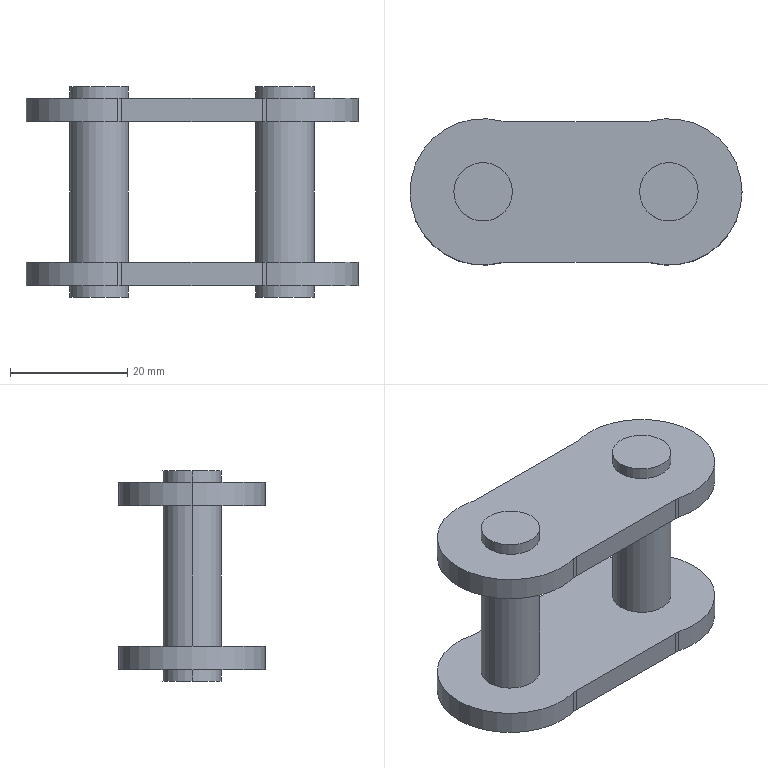Part | STEP file | Motor output chain-06B link 2 | 1 solid | 38 faces | box 56.75 x 25 x 36 mm | volume 14459 mm3 | cylinder 26 | plane 12 | commonest cylinder face diameters 10 x12 6 x8 25 x6
STEP:
#1=CARTESIAN_POINT('',(-20.875,0.,-16.));
#2=VERTEX_POINT('',#1);
#3=CARTESIAN_POINT('',(-10.875,0.,-16.));
#4=VERTEX_POINT('',#3);
#5=CARTESIAN_POINT('',(-15.875,0.,-16.));
#6=DIRECTION('',(0.,0.,-1.));
#7=DIRECTION('',(-1.,0.,0.));
#8=AXIS2_PLACEMENT_3D('',#5,#6,#7);
#9=CIRCLE('',#8,5.);
#10=EDGE_CURVE('',#2,#4,#9,.T.);
#11=ORIENTED_EDGE('',*,*,#10,.T.);
#12=CARTESIAN_POINT('',(-10.875,0.,-18.));
#13=VERTEX_POINT('',#12);
#14=CARTESIAN_POINT('',(-10.875,0.,18.));
#15=DIRECTION('',(0.,0.,-1.));
#16=VECTOR('',#15,1000.);
#17=LINE('',#14,#16);
#18=EDGE_CURVE('',#4,#13,#17,.T.);
#19=ORIENTED_EDGE('',*,*,#18,.T.);
#20=CARTESIAN_POINT('',(-20.875,0.,-18.));
#21=VERTEX_POINT('',#20);
#22=CARTESIAN_POINT('',(-15.875,0.,-18.));
#23=DIRECTION('',(0.,0.,1.));
#24=DIRECTION('',(1.,0.,0.));
#25=AXIS2_PLACEMENT_3D('',#22,#23,#24);
#26=CIRCLE('',#25,5.);
#27=EDGE_CURVE('',#13,#21,#26,.T.);
#28=ORIENTED_EDGE('',*,*,#27,.T.);
#29=CARTESIAN_POINT('',(-20.875,0.,18.));
#30=DIRECTION('',(0.,0.,-1.));
#31=VECTOR('',#30,1000.);
#32=LINE('',#29,#31);
#33=EDGE_CURVE('',#2,#21,#32,.T.);
#34=ORIENTED_EDGE('',*,*,#33,.F.);
#35=EDGE_LOOP('',(#11,#19,#28,#34));
#36=FACE_OUTER_BOUND('',#35,.T.);
#37=CARTESIAN_POINT('',(-15.875,0.,18.));
#38=DIRECTION('',(0.,0.,-1.));
#39=DIRECTION('',(-1.,0.,0.));
#40=AXIS2_PLACEMENT_3D('',#37,#38,#39);
#41=CYLINDRICAL_SURFACE('',#40,5.);
#42=ADVANCED_FACE('',(#36),#41,.T.);
#43=CARTESIAN_POINT('',(10.875,0.,-16.));
#44=VERTEX_POINT('',#43);
#45=CARTESIAN_POINT('',(20.875,0.,-16.));
#46=VERTEX_POINT('',#45);
#47=CARTESIAN_POINT('',(15.875,0.,-16.));
#48=DIRECTION('',(0.,0.,-1.));
#49=DIRECTION('',(-1.,0.,0.));
#50=AXIS2_PLACEMENT_3D('',#47,#48,#49);
#51=CIRCLE('',#50,5.);
#52=EDGE_CURVE('',#44,#46,#51,.T.);
#53=ORIENTED_EDGE('',*,*,#52,.T.);
#54=CARTESIAN_POINT('',(20.875,0.,-18.));
#55=VERTEX_POINT('',#54);
#56=CARTESIAN_POINT('',(20.875,0.,18.));
#57=DIRECTION('',(0.,0.,-1.));
#58=VECTOR('',#57,1000.);
#59=LINE('',#56,#58);
#60=EDGE_CURVE('',#46,#55,#59,.T.);
#61=ORIENTED_EDGE('',*,*,#60,.T.);
#62=CARTESIAN_POINT('',(10.875,0.,-18.));
#63=VERTEX_POINT('',#62);
#64=CARTESIAN_POINT('',(15.875,0.,-18.));
#65=DIRECTION('',(0.,0.,1.));
#66=DIRECTION('',(1.,0.,0.));
#67=AXIS2_PLACEMENT_3D('',#64,#65,#66);
#68=CIRCLE('',#67,5.);
#69=EDGE_CURVE('',#55,#63,#68,.T.);
#70=ORIENTED_EDGE('',*,*,#69,.T.);
#71=CARTESIAN_POINT('',(10.875,0.,18.));
#72=DIRECTION('',(0.,0.,-1.));
#73=VECTOR('',#72,1000.);
#74=LINE('',#71,#73);
#75=EDGE_CURVE('',#44,#63,#74,.T.);
#76=ORIENTED_EDGE('',*,*,#75,.F.);
#77=EDGE_LOOP('',(#53,#61,#70,#76));
#78=FACE_OUTER_BOUND('',#77,.T.);
#79=CARTESIAN_POINT('',(15.875,0.,18.));
#80=DIRECTION('',(0.,0.,-1.));
#81=DIRECTION('',(-1.,0.,0.));
#82=AXIS2_PLACEMENT_3D('',#79,#80,#81);
#83=CYLINDRICAL_SURFACE('',#82,5.);
#84=ADVANCED_FACE('',(#78),#83,.T.);
#85=CARTESIAN_POINT('',(12.726,-12.097,-16.));
#86=VERTEX_POINT('',#85);
#87=CARTESIAN_POINT('',(28.375,0.,-16.));
#88=VERTEX_POINT('',#87);
#89=CARTESIAN_POINT('',(15.875,0.,-16.));
#90=DIRECTION('',(0.,0.,1.));
#91=DIRECTION('',(1.,0.,0.));
#92=AXIS2_PLACEMENT_3D('',#89,#90,#91);
#93=CIRCLE('',#92,12.5);
#94=EDGE_CURVE('',#86,#88,#93,.T.);
#95=ORIENTED_EDGE('',*,*,#94,.T.);
#96=CARTESIAN_POINT('',(28.375,0.,-12.));
#97=VERTEX_POINT('',#96);
#98=CARTESIAN_POINT('',(28.375,0.,-16.));
#99=DIRECTION('',(0.,0.,1.));
#100=VECTOR('',#99,1000.);
#101=LINE('',#98,#100);
#102=EDGE_CURVE('',#88,#97,#101,.T.);
#103=ORIENTED_EDGE('',*,*,#102,.T.);
#104=CARTESIAN_POINT('',(12.726,-12.097,-12.));
#105=VERTEX_POINT('',#104);
#106=CARTESIAN_POINT('',(15.875,0.,-12.));
#107=DIRECTION('',(0.,0.,1.));
#108=DIRECTION('',(1.,0.,0.));
#109=AXIS2_PLACEMENT_3D('',#106,#107,#108);
#110=CIRCLE('',#109,12.5);
#111=EDGE_CURVE('',#105,#97,#110,.T.);
#112=ORIENTED_EDGE('',*,*,#111,.F.);
#113=CARTESIAN_POINT('',(12.726,-12.097,-16.));
#114=DIRECTION('',(0.,0.,1.));
#115=VECTOR('',#114,1000.);
#116=LINE('',#113,#115);
#117=EDGE_CURVE('',#86,#105,#116,.T.);
#118=ORIENTED_EDGE('',*,*,#117,.F.);
#119=EDGE_LOOP('',(#95,#103,#112,#118));
#120=FACE_OUTER_BOUND('',#119,.T.);
#121=CARTESIAN_POINT('',(15.875,0.,-16.));
#122=DIRECTION('',(0.,0.,1.));
#123=DIRECTION('',(1.,0.,0.));
#124=AXIS2_PLACEMENT_3D('',#121,#122,#123);
#125=CYLINDRICAL_SURFACE('',#124,12.5);
#126=ADVANCED_FACE('',(#120),#125,.T.);
#127=CARTESIAN_POINT('',(20.875,0.,18.));
#128=VERTEX_POINT('',#127);
#129=CARTESIAN_POINT('',(10.875,0.,18.));
#130=VERTEX_POINT('',#129);
#131=CARTESIAN_POINT('',(15.875,0.,18.));
#132=DIRECTION('',(0.,0.,1.));
#133=DIRECTION('',(1.,0.,0.));
#134=AXIS2_PLACEMENT_3D('',#131,#132,#133);
#135=CIRCLE('',#134,5.);
#136=EDGE_CURVE('',#128,#130,#135,.T.);
#137=ORIENTED_EDGE('',*,*,#136,.F.);
#138=CARTESIAN_POINT('',(20.875,0.,16.));
#139=VERTEX_POINT('',#138);
#140=CARTESIAN_POINT('',(20.875,0.,18.));
#141=DIRECTION('',(0.,0.,-1.));
#142=VECTOR('',#141,1000.);
#143=LINE('',#140,#142);
#144=EDGE_CURVE('',#128,#139,#143,.T.);
#145=ORIENTED_EDGE('',*,*,#144,.T.);
#146=CARTESIAN_POINT('',(10.875,0.,16.));
#147=VERTEX_POINT('',#146);
#148=CARTESIAN_POINT('',(15.875,0.,16.));
#149=DIRECTION('',(0.,0.,-1.));
#150=DIRECTION('',(1.,0.,0.));
#151=AXIS2_PLACEMENT_3D('',#148,#149,#150);
#152=CIRCLE('',#151,5.);
#153=EDGE_CURVE('',#147,#139,#152,.T.);
#154=ORIENTED_EDGE('',*,*,#153,.F.);
#155=CARTESIAN_POINT('',(10.875,0.,18.));
#156=DIRECTION('',(0.,0.,-1.));
#157=VECTOR('',#156,1000.);
#158=LINE('',#155,#157);
#159=EDGE_CURVE('',#130,#147,#158,.T.);
#160=ORIENTED_EDGE('',*,*,#159,.F.);
#161=EDGE_LOOP('',(#137,#145,#154,#160));
#162=FACE_OUTER_BOUND('',#161,.T.);
#163=CARTESIAN_POINT('',(15.875,0.,18.));
#164=DIRECTION('',(0.,0.,-1.));
#165=DIRECTION('',(-1.,0.,0.));
#166=AXIS2_PLACEMENT_3D('',#163,#164,#165);
#167=CYLINDRICAL_SURFACE('',#166,5.);
#168=ADVANCED_FACE('',(#162),#167,.T.);
#169=CARTESIAN_POINT('',(-28.375,0.,16.));
#170=VERTEX_POINT('',#169);
#171=CARTESIAN_POINT('',(-12.726,-12.097,16.));
#172=VERTEX_POINT('',#171);
#173=CARTESIAN_POINT('',(-15.875,0.,16.));
#174=DIRECTION('',(0.,0.,1.));
#175=DIRECTION('',(1.,0.,0.));
#176=AXIS2_PLACEMENT_3D('',#173,#174,#175);
#177=CIRCLE('',#176,12.5);
#178=EDGE_CURVE('',#170,#172,#177,.T.);
#179=ORIENTED_EDGE('',*,*,#178,.F.);
#180=CARTESIAN_POINT('',(-28.375,0.,12.));
#181=VERTEX_POINT('',#180);
#182=CARTESIAN_POINT('',(-28.375,0.,16.));
#183=DIRECTION('',(0.,0.,-1.));
#184=VECTOR('',#183,1000.);
#185=LINE('',#182,#184);
#186=EDGE_CURVE('',#170,#181,#185,.T.);
#187=ORIENTED_EDGE('',*,*,#186,.T.);
#188=CARTESIAN_POINT('',(-12.726,-12.097,12.));
#189=VERTEX_POINT('',#188);
#190=CARTESIAN_POINT('',(-15.875,0.,12.));
#191=DIRECTION('',(0.,0.,1.));
#192=DIRECTION('',(1.,0.,0.));
#193=AXIS2_PLACEMENT_3D('',#190,#191,#192);
#194=CIRCLE('',#193,12.5);
#195=EDGE_CURVE('',#181,#189,#194,.T.);
#196=ORIENTED_EDGE('',*,*,#195,.T.);
#197=CARTESIAN_POINT('',(-12.726,-12.097,16.));
#198=DIRECTION('',(0.,0.,-1.));
#199=VECTOR('',#198,1000.);
#200=LINE('',#197,#199);
#201=EDGE_CURVE('',#172,#189,#200,.T.);
#202=ORIENTED_EDGE('',*,*,#201,.F.);
#203=EDGE_LOOP('',(#179,#187,#196,#202));
#204=FACE_OUTER_BOUND('',#203,.T.);
#205=CARTESIAN_POINT('',(-15.875,0.,16.));
#206=DIRECTION('',(0.,0.,-1.));
#207=DIRECTION('',(-1.,0.,0.));
#208=AXIS2_PLACEMENT_3D('',#205,#206,#207);
#209=CYLINDRICAL_SURFACE('',#208,12.5);
#210=ADVANCED_FACE('',(#204),#209,.T.);
#211=CARTESIAN_POINT('',(-10.875,0.,18.));
#212=VERTEX_POINT('',#211);
#213=CARTESIAN_POINT('',(-20.875,0.,18.));
#214=VERTEX_POINT('',#213);
#215=CARTESIAN_POINT('',(-15.875,0.,18.));
#216=DIRECTION('',(0.,0.,1.));
#217=DIRECTION('',(1.,0.,0.));
#218=AXIS2_PLACEMENT_3D('',#215,#216,#217);
#219=CIRCLE('',#218,5.);
#220=EDGE_CURVE('',#212,#214,#219,.T.);
#221=ORIENTED_EDGE('',*,*,#220,.F.);
#222=CARTESIAN_POINT('',(-10.875,0.,16.));
#223=VERTEX_POINT('',#222);
#224=CARTESIAN_POINT('',(-10.875,0.,18.));
#225=DIRECTION('',(0.,0.,-1.));
#226=VECTOR('',#225,1000.);
#227=LINE('',#224,#226);
#228=EDGE_CURVE('',#212,#223,#227,.T.);
#229=ORIENTED_EDGE('',*,*,#228,.T.);
#230=CARTESIAN_POINT('',(-20.875,0.,16.));
#231=VERTEX_POINT('',#230);
#232=CARTESIAN_POINT('',(-15.875,0.,16.));
#233=DIRECTION('',(0.,0.,1.));
#234=DIRECTION('',(1.,0.,0.));
#235=AXIS2_PLACEMENT_3D('',#232,#233,#234);
#236=CIRCLE('',#235,5.);
#237=EDGE_CURVE('',#223,#231,#236,.T.);
#238=ORIENTED_EDGE('',*,*,#237,.T.);
#239=CARTESIAN_POINT('',(-20.875,0.,18.));
#240=DIRECTION('',(0.,0.,-1.));
#241=VECTOR('',#240,1000.);
#242=LINE('',#239,#241);
#243=EDGE_CURVE('',#214,#231,#242,.T.);
#244=ORIENTED_EDGE('',*,*,#243,.F.);
#245=EDGE_LOOP('',(#221,#229,#238,#244));
#246=FACE_OUTER_BOUND('',#245,.T.);
#247=CARTESIAN_POINT('',(-15.875,0.,18.));
#248=DIRECTION('',(0.,0.,-1.));
#249=DIRECTION('',(-1.,0.,0.));
#250=AXIS2_PLACEMENT_3D('',#247,#248,#249);
#251=CYLINDRICAL_SURFACE('',#250,5.);
#252=ADVANCED_FACE('',(#246),#251,.T.);
#253=CARTESIAN_POINT('',(10.875,0.,12.));
#254=VERTEX_POINT('',#253);
#255=CARTESIAN_POINT('',(20.875,0.,12.));
#256=VERTEX_POINT('',#255);
#257=CARTESIAN_POINT('',(15.875,0.,12.));
#258=DIRECTION('',(0.,0.,-1.));
#259=DIRECTION('',(1.,0.,0.));
#260=AXIS2_PLACEMENT_3D('',#257,#258,#259);
#261=CIRCLE('',#260,5.);
#262=EDGE_CURVE('',#254,#256,#261,.T.);
#263=ORIENTED_EDGE('',*,*,#262,.T.);
#264=CARTESIAN_POINT('',(20.875,0.,-12.));
#265=VERTEX_POINT('',#264);
#266=CARTESIAN_POINT('',(20.875,0.,18.));
#267=DIRECTION('',(0.,0.,-1.));
#268=VECTOR('',#267,1000.);
#269=LINE('',#266,#268);
#270=EDGE_CURVE('',#256,#265,#269,.T.);
#271=ORIENTED_EDGE('',*,*,#270,.T.);
#272=CARTESIAN_POINT('',(10.875,0.,-12.));
#273=VERTEX_POINT('',#272);
#274=CARTESIAN_POINT('',(15.875,0.,-12.));
#275=DIRECTION('',(0.,0.,-1.));
#276=DIRECTION('',(-1.,0.,0.));
#277=AXIS2_PLACEMENT_3D('',#274,#275,#276);
#278=CIRCLE('',#277,5.);
#279=EDGE_CURVE('',#273,#265,#278,.T.);
#280=ORIENTED_EDGE('',*,*,#279,.F.);
#281=CARTESIAN_POINT('',(10.875,0.,18.));
#282=DIRECTION('',(0.,0.,-1.));
#283=VECTOR('',#282,1000.);
#284=LINE('',#281,#283);
#285=EDGE_CURVE('',#254,#273,#284,.T.);
#286=ORIENTED_EDGE('',*,*,#285,.F.);
#287=EDGE_LOOP('',(#263,#271,#280,#286));
#288=FACE_OUTER_BOUND('',#287,.T.);
#289=CARTESIAN_POINT('',(15.875,0.,18.));
#290=DIRECTION('',(0.,0.,-1.));
#291=DIRECTION('',(-1.,0.,0.));
#292=AXIS2_PLACEMENT_3D('',#289,#290,#291);
#293=CYLINDRICAL_SURFACE('',#292,5.);
#294=ADVANCED_FACE('',(#288),#293,.T.);
#295=CARTESIAN_POINT('',(-10.875,0.,12.));
#296=VERTEX_POINT('',#295);
#297=CARTESIAN_POINT('',(-20.875,0.,12.));
#298=VERTEX_POINT('',#297);
#299=CARTESIAN_POINT('',(-15.875,0.,12.));
#300=DIRECTION('',(0.,0.,1.));
#301=DIRECTION('',(1.,0.,0.));
#302=AXIS2_PLACEMENT_3D('',#299,#300,#301);
#303=CIRCLE('',#302,5.);
#304=EDGE_CURVE('',#296,#298,#303,.T.);
#305=ORIENTED_EDGE('',*,*,#304,.F.);
#306=CARTESIAN_POINT('',(-10.875,0.,-12.));
#307=VERTEX_POINT('',#306);
#308=CARTESIAN_POINT('',(-10.875,0.,18.));
#309=DIRECTION('',(0.,0.,-1.));
#310=VECTOR('',#309,1000.);
#311=LINE('',#308,#310);
#312=EDGE_CURVE('',#296,#307,#311,.T.);
#313=ORIENTED_EDGE('',*,*,#312,.T.);
#314=CARTESIAN_POINT('',(-20.875,0.,-12.));
#315=VERTEX_POINT('',#314);
#316=CARTESIAN_POINT('',(-15.875,0.,-12.));
#317=DIRECTION('',(0.,0.,-1.));
#318=DIRECTION('',(-1.,0.,0.));
#319=AXIS2_PLACEMENT_3D('',#316,#317,#318);
#320=CIRCLE('',#319,5.);
#321=EDGE_CURVE('',#315,#307,#320,.T.);
#322=ORIENTED_EDGE('',*,*,#321,.F.);
#323=CARTESIAN_POINT('',(-20.875,0.,18.));
#324=DIRECTION('',(0.,0.,-1.));
#325=VECTOR('',#324,1000.);
#326=LINE('',#323,#325);
#327=EDGE_CURVE('',#298,#315,#326,.T.);
#328=ORIENTED_EDGE('',*,*,#327,.F.);
#329=EDGE_LOOP('',(#305,#313,#322,#328));
#330=FACE_OUTER_BOUND('',#329,.T.);
#331=CARTESIAN_POINT('',(-15.875,0.,18.));
#332=DIRECTION('',(0.,0.,-1.));
#333=DIRECTION('',(-1.,0.,0.));
#334=AXIS2_PLACEMENT_3D('',#331,#332,#333);
#335=CYLINDRICAL_SURFACE('',#334,5.);
#336=ADVANCED_FACE('',(#330),#335,.T.);
#337=ORIENTED_EDGE('',*,*,#312,.F.);
#338=CARTESIAN_POINT('',(-15.875,0.,12.));
#339=DIRECTION('',(0.,0.,1.));
#340=DIRECTION('',(1.,0.,0.));
#341=AXIS2_PLACEMENT_3D('',#338,#339,#340);
#342=CIRCLE('',#341,5.);
#343=EDGE_CURVE('',#298,#296,#342,.T.);
#344=ORIENTED_EDGE('',*,*,#343,.F.);
#345=ORIENTED_EDGE('',*,*,#327,.T.);
#346=CARTESIAN_POINT('',(-15.875,0.,-12.));
#347=DIRECTION('',(0.,0.,-1.));
#348=DIRECTION('',(-1.,0.,0.));
#349=AXIS2_PLACEMENT_3D('',#346,#347,#348);
#350=CIRCLE('',#349,5.);
#351=EDGE_CURVE('',#307,#315,#350,.T.);
#352=ORIENTED_EDGE('',*,*,#351,.F.);
#353=EDGE_LOOP('',(#337,#344,#345,#352));
#354=FACE_OUTER_BOUND('',#353,.T.);
#355=CARTESIAN_POINT('',(-15.875,0.,18.));
#356=DIRECTION('',(0.,0.,-1.));
#357=DIRECTION('',(-1.,0.,0.));
#358=AXIS2_PLACEMENT_3D('',#355,#356,#357);
#359=CYLINDRICAL_SURFACE('',#358,5.);
#360=ADVANCED_FACE('',(#354),#359,.T.);
#361=ORIENTED_EDGE('',*,*,#270,.F.);
#362=CARTESIAN_POINT('',(15.875,0.,12.));
#363=DIRECTION('',(0.,0.,-1.));
#364=DIRECTION('',(1.,0.,0.));
#365=AXIS2_PLACEMENT_3D('',#362,#363,#364);
#366=CIRCLE('',#365,5.);
#367=EDGE_CURVE('',#256,#254,#366,.T.);
#368=ORIENTED_EDGE('',*,*,#367,.T.);
#369=ORIENTED_EDGE('',*,*,#285,.T.);
#370=CARTESIAN_POINT('',(15.875,0.,-12.));
#371=DIRECTION('',(0.,0.,-1.));
#372=DIRECTION('',(-1.,0.,0.));
#373=AXIS2_PLACEMENT_3D('',#370,#371,#372);
#374=CIRCLE('',#373,5.);
#375=EDGE_CURVE('',#265,#273,#374,.T.);
#376=ORIENTED_EDGE('',*,*,#375,.F.);
#377=EDGE_LOOP('',(#361,#368,#369,#376));
#378=FACE_OUTER_BOUND('',#377,.T.);
#379=CARTESIAN_POINT('',(15.875,0.,18.));
#380=DIRECTION('',(0.,0.,-1.));
#381=DIRECTION('',(-1.,0.,0.));
#382=AXIS2_PLACEMENT_3D('',#379,#380,#381);
#383=CYLINDRICAL_SURFACE('',#382,5.);
#384=ADVANCED_FACE('',(#378),#383,.T.);
#385=ORIENTED_EDGE('',*,*,#228,.F.);
#386=CARTESIAN_POINT('',(-15.875,0.,18.));
#387=DIRECTION('',(0.,0.,1.));
#388=DIRECTION('',(1.,0.,0.));
#389=AXIS2_PLACEMENT_3D('',#386,#387,#388);
#390=CIRCLE('',#389,5.);
#391=EDGE_CURVE('',#214,#212,#390,.T.);
#392=ORIENTED_EDGE('',*,*,#391,.F.);
#393=ORIENTED_EDGE('',*,*,#243,.T.);
#394=CARTESIAN_POINT('',(-15.875,0.,16.));
#395=DIRECTION('',(0.,0.,1.));
#396=DIRECTION('',(1.,0.,0.));
#397=AXIS2_PLACEMENT_3D('',#394,#395,#396);
#398=CIRCLE('',#397,5.);
#399=EDGE_CURVE('',#231,#223,#398,.T.);
#400=ORIENTED_EDGE('',*,*,#399,.T.);
#401=EDGE_LOOP('',(#385,#392,#393,#400));
#402=FACE_OUTER_BOUND('',#401,.T.);
#403=CARTESIAN_POINT('',(-15.875,0.,18.));
#404=DIRECTION('',(0.,0.,-1.));
#405=DIRECTION('',(-1.,0.,0.));
#406=AXIS2_PLACEMENT_3D('',#403,#404,#405);
#407=CYLINDRICAL_SURFACE('',#406,5.);
#408=ADVANCED_FACE('',(#402),#407,.T.);
#409=ORIENTED_EDGE('',*,*,#391,.T.);
#410=ORIENTED_EDGE('',*,*,#220,.T.);
#411=EDGE_LOOP('',(#409,#410));
#412=FACE_OUTER_BOUND('',#411,.T.);
#413=CARTESIAN_POINT('',(-15.875,0.,18.));
#414=DIRECTION('',(0.,0.,1.));
#415=DIRECTION('',(1.,0.,0.));
#416=AXIS2_PLACEMENT_3D('',#413,#414,#415);
#417=PLANE('',#416);
#418=ADVANCED_FACE('',(#412),#417,.T.);
#419=CARTESIAN_POINT('',(-11.97,-12.,12.));
#420=VERTEX_POINT('',#419);
#421=CARTESIAN_POINT('',(-11.97,-15.,12.));
#422=DIRECTION('',(0.,0.,-1.));
#423=DIRECTION('',(1.,0.,0.));
#424=AXIS2_PLACEMENT_3D('',#421,#422,#423);
#425=CIRCLE('',#424,3.);
#426=EDGE_CURVE('',#189,#420,#425,.T.);
#427=ORIENTED_EDGE('',*,*,#426,.T.);
#428=CARTESIAN_POINT('',(-11.97,-12.,16.));
#429=VERTEX_POINT('',#428);
#430=CARTESIAN_POINT('',(-11.97,-12.,16.));
#431=DIRECTION('',(0.,0.,-1.));
#432=VECTOR('',#431,1000.);
#433=LINE('',#430,#432);
#434=EDGE_CURVE('',#429,#420,#433,.T.);
#435=ORIENTED_EDGE('',*,*,#434,.F.);
#436=CARTESIAN_POINT('',(-11.97,-15.,16.));
#437=DIRECTION('',(0.,0.,-1.));
#438=DIRECTION('',(1.,0.,0.));
#439=AXIS2_PLACEMENT_3D('',#436,#437,#438);
#440=CIRCLE('',#439,3.);
#441=EDGE_CURVE('',#172,#429,#440,.T.);
#442=ORIENTED_EDGE('',*,*,#441,.F.);
#443=ORIENTED_EDGE('',*,*,#201,.T.);
#444=EDGE_LOOP('',(#427,#435,#442,#443));
#445=FACE_OUTER_BOUND('',#444,.T.);
#446=CARTESIAN_POINT('',(-11.97,-15.,16.));
#447=DIRECTION('',(0.,0.,-1.));
#448=DIRECTION('',(-1.,0.,0.));
#449=AXIS2_PLACEMENT_3D('',#446,#447,#448);
#450=CYLINDRICAL_SURFACE('',#449,3.);
#451=ADVANCED_FACE('',(#445),#450,.F.);
#452=CARTESIAN_POINT('',(11.97,-12.,12.));
#453=VERTEX_POINT('',#452);
#454=CARTESIAN_POINT('',(-11.97,-12.,12.));
#455=DIRECTION('',(1.,0.,0.));
#456=VECTOR('',#455,1000.);
#457=LINE('',#454,#456);
#458=EDGE_CURVE('',#420,#453,#457,.T.);
#459=ORIENTED_EDGE('',*,*,#458,.T.);
#460=CARTESIAN_POINT('',(11.97,-12.,16.));
#461=VERTEX_POINT('',#460);
#462=CARTESIAN_POINT('',(11.97,-12.,16.));
#463=DIRECTION('',(0.,0.,-1.));
#464=VECTOR('',#463,1000.);
#465=LINE('',#462,#464);
#466=EDGE_CURVE('',#461,#453,#465,.T.);
#467=ORIENTED_EDGE('',*,*,#466,.F.);
#468=CARTESIAN_POINT('',(-11.97,-12.,16.));
#469=DIRECTION('',(1.,0.,0.));
#470=VECTOR('',#469,1000.);
#471=LINE('',#468,#470);
#472=EDGE_CURVE('',#429,#461,#471,.T.);
#473=ORIENTED_EDGE('',*,*,#472,.F.);
#474=ORIENTED_EDGE('',*,*,#434,.T.);
#475=EDGE_LOOP('',(#459,#467,#473,#474));
#476=FACE_OUTER_BOUND('',#475,.T.);
#477=CARTESIAN_POINT('',(-11.97,-12.,16.));
#478=DIRECTION('',(0.,1.,0.));
#479=DIRECTION('',(0.,0.,1.));
#480=AXIS2_PLACEMENT_3D('',#477,#478,#479);
#481=PLANE('',#480);
#482=ADVANCED_FACE('',(#476),#481,.F.);
#483=CARTESIAN_POINT('',(12.726,-12.097,12.));
#484=VERTEX_POINT('',#483);
#485=CARTESIAN_POINT('',(11.97,-15.,12.));
#486=DIRECTION('',(0.,0.,-1.));
#487=DIRECTION('',(-1.,0.,0.));
#488=AXIS2_PLACEMENT_3D('',#485,#486,#487);
#489=CIRCLE('',#488,3.);
#490=EDGE_CURVE('',#453,#484,#489,.T.);
#491=ORIENTED_EDGE('',*,*,#490,.T.);
#492=CARTESIAN_POINT('',(12.726,-12.097,16.));
#493=VERTEX_POINT('',#492);
#494=CARTESIAN_POINT('',(12.726,-12.097,16.));
#495=DIRECTION('',(0.,0.,-1.));
#496=VECTOR('',#495,1000.);
#497=LINE('',#494,#496);
#498=EDGE_CURVE('',#493,#484,#497,.T.);
#499=ORIENTED_EDGE('',*,*,#498,.F.);
#500=CARTESIAN_POINT('',(11.97,-15.,16.));
#501=DIRECTION('',(0.,0.,-1.));
#502=DIRECTION('',(-1.,0.,0.));
#503=AXIS2_PLACEMENT_3D('',#500,#501,#502);
#504=CIRCLE('',#503,3.);
#505=EDGE_CURVE('',#461,#493,#504,.T.);
#506=ORIENTED_EDGE('',*,*,#505,.F.);
#507=ORIENTED_EDGE('',*,*,#466,.T.);
#508=EDGE_LOOP('',(#491,#499,#506,#507));
#509=FACE_OUTER_BOUND('',#508,.T.);
#510=CARTESIAN_POINT('',(11.97,-15.,16.));
#511=DIRECTION('',(0.,0.,-1.));
#512=DIRECTION('',(-1.,0.,0.));
#513=AXIS2_PLACEMENT_3D('',#510,#511,#512);
#514=CYLINDRICAL_SURFACE('',#513,3.);
#515=ADVANCED_FACE('',(#509),#514,.F.);
#516=CARTESIAN_POINT('',(12.726,12.097,12.));
#517=VERTEX_POINT('',#516);
#518=CARTESIAN_POINT('',(15.875,0.,12.));
#519=DIRECTION('',(0.,0.,1.));
#520=DIRECTION('',(1.,0.,0.));
#521=AXIS2_PLACEMENT_3D('',#518,#519,#520);
#522=CIRCLE('',#521,12.5);
#523=EDGE_CURVE('',#484,#517,#522,.T.);
#524=ORIENTED_EDGE('',*,*,#523,.T.);
#525=CARTESIAN_POINT('',(12.726,12.097,16.));
#526=VERTEX_POINT('',#525);
#527=CARTESIAN_POINT('',(12.726,12.097,16.));
#528=DIRECTION('',(0.,0.,-1.));
#529=VECTOR('',#528,1000.);
#530=LINE('',#527,#529);
#531=EDGE_CURVE('',#526,#517,#530,.T.);
#532=ORIENTED_EDGE('',*,*,#531,.F.);
#533=CARTESIAN_POINT('',(15.875,0.,16.));
#534=DIRECTION('',(0.,0.,1.));
#535=DIRECTION('',(1.,0.,0.));
#536=AXIS2_PLACEMENT_3D('',#533,#534,#535);
#537=CIRCLE('',#536,12.5);
#538=EDGE_CURVE('',#493,#526,#537,.T.);
#539=ORIENTED_EDGE('',*,*,#538,.F.);
#540=ORIENTED_EDGE('',*,*,#498,.T.);
#541=EDGE_LOOP('',(#524,#532,#539,#540));
#542=FACE_OUTER_BOUND('',#541,.T.);
#543=CARTESIAN_POINT('',(15.875,0.,16.));
#544=DIRECTION('',(0.,0.,-1.));
#545=DIRECTION('',(-1.,0.,0.));
#546=AXIS2_PLACEMENT_3D('',#543,#544,#545);
#547=CYLINDRICAL_SURFACE('',#546,12.5);
#548=ADVANCED_FACE('',(#542),#547,.T.);
#549=CARTESIAN_POINT('',(11.97,12.,12.));
#550=VERTEX_POINT('',#549);
#551=CARTESIAN_POINT('',(11.97,15.,12.));
#552=DIRECTION('',(0.,0.,-1.));
#553=DIRECTION('',(1.,0.,0.));
#554=AXIS2_PLACEMENT_3D('',#551,#552,#553);
#555=CIRCLE('',#554,3.);
#556=EDGE_CURVE('',#517,#550,#555,.T.);
#557=ORIENTED_EDGE('',*,*,#556,.T.);
#558=CARTESIAN_POINT('',(11.97,12.,16.));
#559=VERTEX_POINT('',#558);
#560=CARTESIAN_POINT('',(11.97,12.,16.));
#561=DIRECTION('',(0.,0.,-1.));
#562=VECTOR('',#561,1000.);
#563=LINE('',#560,#562);
#564=EDGE_CURVE('',#559,#550,#563,.T.);
#565=ORIENTED_EDGE('',*,*,#564,.F.);
#566=CARTESIAN_POINT('',(11.97,15.,16.));
#567=DIRECTION('',(0.,0.,-1.));
#568=DIRECTION('',(1.,0.,0.));
#569=AXIS2_PLACEMENT_3D('',#566,#567,#568);
#570=CIRCLE('',#569,3.);
#571=EDGE_CURVE('',#526,#559,#570,.T.);
#572=ORIENTED_EDGE('',*,*,#571,.F.);
#573=ORIENTED_EDGE('',*,*,#531,.T.);
#574=EDGE_LOOP('',(#557,#565,#572,#573));
#575=FACE_OUTER_BOUND('',#574,.T.);
#576=CARTESIAN_POINT('',(11.97,15.,16.));
#577=DIRECTION('',(0.,0.,-1.));
#578=DIRECTION('',(-1.,0.,0.));
#579=AXIS2_PLACEMENT_3D('',#576,#577,#578);
#580=CYLINDRICAL_SURFACE('',#579,3.);
#581=ADVANCED_FACE('',(#575),#580,.F.);
#582=CARTESIAN_POINT('',(-11.97,12.,12.));
#583=VERTEX_POINT('',#582);
#584=CARTESIAN_POINT('',(-11.97,12.,12.));
#585=DIRECTION('',(-1.,0.,0.));
#586=VECTOR('',#585,1000.);
#587=LINE('',#584,#586);
#588=EDGE_CURVE('',#550,#583,#587,.T.);
#589=ORIENTED_EDGE('',*,*,#588,.T.);
#590=CARTESIAN_POINT('',(-11.97,12.,16.));
#591=VERTEX_POINT('',#590);
#592=CARTESIAN_POINT('',(-11.97,12.,16.));
#593=DIRECTION('',(0.,0.,-1.));
#594=VECTOR('',#593,1000.);
#595=LINE('',#592,#594);
#596=EDGE_CURVE('',#591,#583,#595,.T.);
#597=ORIENTED_EDGE('',*,*,#596,.F.);
#598=CARTESIAN_POINT('',(-11.97,12.,16.));
#599=DIRECTION('',(-1.,0.,0.));
#600=VECTOR('',#599,1000.);
#601=LINE('',#598,#600);
#602=EDGE_CURVE('',#559,#591,#601,.T.);
#603=ORIENTED_EDGE('',*,*,#602,.F.);
#604=ORIENTED_EDGE('',*,*,#564,.T.);
#605=EDGE_LOOP('',(#589,#597,#603,#604));
#606=FACE_OUTER_BOUND('',#605,.T.);
#607=CARTESIAN_POINT('',(-11.97,12.,16.));
#608=DIRECTION('',(0.,-1.,0.));
#609=DIRECTION('',(0.,0.,-1.));
#610=AXIS2_PLACEMENT_3D('',#607,#608,#609);
#611=PLANE('',#610);
#612=ADVANCED_FACE('',(#606),#611,.F.);
#613=CARTESIAN_POINT('',(-12.726,12.097,12.));
#614=VERTEX_POINT('',#613);
#615=CARTESIAN_POINT('',(-11.97,15.,12.));
#616=DIRECTION('',(0.,0.,-1.));
#617=DIRECTION('',(-1.,0.,0.));
#618=AXIS2_PLACEMENT_3D('',#615,#616,#617);
#619=CIRCLE('',#618,3.);
#620=EDGE_CURVE('',#583,#614,#619,.T.);
#621=ORIENTED_EDGE('',*,*,#620,.T.);
#622=CARTESIAN_POINT('',(-12.726,12.097,16.));
#623=VERTEX_POINT('',#622);
#624=CARTESIAN_POINT('',(-12.726,12.097,16.));
#625=DIRECTION('',(0.,0.,-1.));
#626=VECTOR('',#625,1000.);
#627=LINE('',#624,#626);
#628=EDGE_CURVE('',#623,#614,#627,.T.);
#629=ORIENTED_EDGE('',*,*,#628,.F.);
#630=CARTESIAN_POINT('',(-11.97,15.,16.));
#631=DIRECTION('',(0.,0.,-1.));
#632=DIRECTION('',(-1.,0.,0.));
#633=AXIS2_PLACEMENT_3D('',#630,#631,#632);
#634=CIRCLE('',#633,3.);
#635=EDGE_CURVE('',#591,#623,#634,.T.);
#636=ORIENTED_EDGE('',*,*,#635,.F.);
#637=ORIENTED_EDGE('',*,*,#596,.T.);
#638=EDGE_LOOP('',(#621,#629,#636,#637));
#639=FACE_OUTER_BOUND('',#638,.T.);
#640=CARTESIAN_POINT('',(-11.97,15.,16.));
#641=DIRECTION('',(0.,0.,-1.));
#642=DIRECTION('',(-1.,0.,0.));
#643=AXIS2_PLACEMENT_3D('',#640,#641,#642);
#644=CYLINDRICAL_SURFACE('',#643,3.);
#645=ADVANCED_FACE('',(#639),#644,.F.);
#646=ORIENTED_EDGE('',*,*,#186,.F.);
#647=CARTESIAN_POINT('',(-15.875,0.,16.));
#648=DIRECTION('',(0.,0.,1.));
#649=DIRECTION('',(1.,0.,0.));
#650=AXIS2_PLACEMENT_3D('',#647,#648,#649);
#651=CIRCLE('',#650,12.5);
#652=EDGE_CURVE('',#623,#170,#651,.T.);
#653=ORIENTED_EDGE('',*,*,#652,.F.);
#654=ORIENTED_EDGE('',*,*,#628,.T.);
#655=CARTESIAN_POINT('',(-15.875,0.,12.));
#656=DIRECTION('',(0.,0.,1.));
#657=DIRECTION('',(1.,0.,0.));
#658=AXIS2_PLACEMENT_3D('',#655,#656,#657);
#659=CIRCLE('',#658,12.5);
#660=EDGE_CURVE('',#614,#181,#659,.T.);
#661=ORIENTED_EDGE('',*,*,#660,.T.);
#662=EDGE_LOOP('',(#646,#653,#654,#661));
#663=FACE_OUTER_BOUND('',#662,.T.);
#664=CARTESIAN_POINT('',(-15.875,0.,16.));
#665=DIRECTION('',(0.,0.,-1.));
#666=DIRECTION('',(-1.,0.,0.));
#667=AXIS2_PLACEMENT_3D('',#664,#665,#666);
#668=CYLINDRICAL_SURFACE('',#667,12.5);
#669=ADVANCED_FACE('',(#663),#668,.T.);
#670=ORIENTED_EDGE('',*,*,#153,.T.);
#671=CARTESIAN_POINT('',(15.875,0.,16.));
#672=DIRECTION('',(0.,0.,-1.));
#673=DIRECTION('',(1.,0.,0.));
#674=AXIS2_PLACEMENT_3D('',#671,#672,#673);
#675=CIRCLE('',#674,5.);
#676=EDGE_CURVE('',#139,#147,#675,.T.);
#677=ORIENTED_EDGE('',*,*,#676,.T.);
#678=EDGE_LOOP('',(#670,#677));
#679=FACE_BOUND('',#678,.T.);
#680=ORIENTED_EDGE('',*,*,#399,.F.);
#681=ORIENTED_EDGE('',*,*,#237,.F.);
#682=EDGE_LOOP('',(#680,#681));
#683=FACE_BOUND('',#682,.T.);
#684=ORIENTED_EDGE('',*,*,#441,.T.);
#685=ORIENTED_EDGE('',*,*,#472,.T.);
#686=ORIENTED_EDGE('',*,*,#505,.T.);
#687=ORIENTED_EDGE('',*,*,#538,.T.);
#688=ORIENTED_EDGE('',*,*,#571,.T.);
#689=ORIENTED_EDGE('',*,*,#602,.T.);
#690=ORIENTED_EDGE('',*,*,#635,.T.);
#691=ORIENTED_EDGE('',*,*,#652,.T.);
#692=ORIENTED_EDGE('',*,*,#178,.T.);
#693=EDGE_LOOP('',(#684,#685,#686,#687,#688,#689,#690,#691,#692));
#694=FACE_OUTER_BOUND('',#693,.T.);
#695=CARTESIAN_POINT('',(-11.97,-15.,16.));
#696=DIRECTION('',(0.,0.,1.));
#697=DIRECTION('',(1.,0.,0.));
#698=AXIS2_PLACEMENT_3D('',#695,#696,#697);
#699=PLANE('',#698);
#700=ADVANCED_FACE('',(#679,#683,#694),#699,.T.);
#701=ORIENTED_EDGE('',*,*,#262,.F.);
#702=ORIENTED_EDGE('',*,*,#367,.F.);
#703=EDGE_LOOP('',(#701,#702));
#704=FACE_BOUND('',#703,.T.);
#705=ORIENTED_EDGE('',*,*,#343,.T.);
#706=ORIENTED_EDGE('',*,*,#304,.T.);
#707=EDGE_LOOP('',(#705,#706));
#708=FACE_BOUND('',#707,.T.);
#709=ORIENTED_EDGE('',*,*,#426,.F.);
#710=ORIENTED_EDGE('',*,*,#195,.F.);
#711=ORIENTED_EDGE('',*,*,#660,.F.);
#712=ORIENTED_EDGE('',*,*,#620,.F.);
#713=ORIENTED_EDGE('',*,*,#588,.F.);
#714=ORIENTED_EDGE('',*,*,#556,.F.);
#715=ORIENTED_EDGE('',*,*,#523,.F.);
#716=ORIENTED_EDGE('',*,*,#490,.F.);
#717=ORIENTED_EDGE('',*,*,#458,.F.);
#718=EDGE_LOOP('',(#709,#710,#711,#712,#713,#714,#715,#716,#717));
#719=FACE_OUTER_BOUND('',#718,.T.);
#720=CARTESIAN_POINT('',(-11.97,-15.,12.));
#721=DIRECTION('',(0.,0.,1.));
#722=DIRECTION('',(1.,0.,0.));
#723=AXIS2_PLACEMENT_3D('',#720,#721,#722);
#724=PLANE('',#723);
#725=ADVANCED_FACE('',(#704,#708,#719),#724,.F.);
#726=ORIENTED_EDGE('',*,*,#144,.F.);
#727=CARTESIAN_POINT('',(15.875,0.,18.));
#728=DIRECTION('',(0.,0.,1.));
#729=DIRECTION('',(1.,0.,0.));
#730=AXIS2_PLACEMENT_3D('',#727,#728,#729);
#731=CIRCLE('',#730,5.);
#732=EDGE_CURVE('',#130,#128,#731,.T.);
#733=ORIENTED_EDGE('',*,*,#732,.F.);
#734=ORIENTED_EDGE('',*,*,#159,.T.);
#735=ORIENTED_EDGE('',*,*,#676,.F.);
#736=EDGE_LOOP('',(#726,#733,#734,#735));
#737=FACE_OUTER_BOUND('',#736,.T.);
#738=CARTESIAN_POINT('',(15.875,0.,18.));
#739=DIRECTION('',(0.,0.,-1.));
#740=DIRECTION('',(-1.,0.,0.));
#741=AXIS2_PLACEMENT_3D('',#738,#739,#740);
#742=CYLINDRICAL_SURFACE('',#741,5.);
#743=ADVANCED_FACE('',(#737),#742,.T.);
#744=ORIENTED_EDGE('',*,*,#732,.T.);
#745=ORIENTED_EDGE('',*,*,#136,.T.);
#746=EDGE_LOOP('',(#744,#745));
#747=FACE_OUTER_BOUND('',#746,.T.);
#748=CARTESIAN_POINT('',(15.875,0.,18.));
#749=DIRECTION('',(0.,0.,1.));
#750=DIRECTION('',(1.,0.,0.));
#751=AXIS2_PLACEMENT_3D('',#748,#749,#750);
#752=PLANE('',#751);
#753=ADVANCED_FACE('',(#747),#752,.T.);
#754=CARTESIAN_POINT('',(-12.726,-12.097,-12.));
#755=VERTEX_POINT('',#754);
#756=CARTESIAN_POINT('',(-11.97,-12.,-12.));
#757=VERTEX_POINT('',#756);
#758=CARTESIAN_POINT('',(-11.97,-15.,-12.));
#759=DIRECTION('',(0.,0.,-1.));
#760=DIRECTION('',(1.,0.,0.));
#761=AXIS2_PLACEMENT_3D('',#758,#759,#760);
#762=CIRCLE('',#761,3.);
#763=EDGE_CURVE('',#755,#757,#762,.T.);
#764=ORIENTED_EDGE('',*,*,#763,.F.);
#765=CARTESIAN_POINT('',(-12.726,-12.097,-16.));
#766=VERTEX_POINT('',#765);
#767=CARTESIAN_POINT('',(-12.726,-12.097,-16.));
#768=DIRECTION('',(0.,0.,1.));
#769=VECTOR('',#768,1000.);
#770=LINE('',#767,#769);
#771=EDGE_CURVE('',#766,#755,#770,.T.);
#772=ORIENTED_EDGE('',*,*,#771,.F.);
#773=CARTESIAN_POINT('',(-11.97,-12.,-16.));
#774=VERTEX_POINT('',#773);
#775=CARTESIAN_POINT('',(-11.97,-15.,-16.));
#776=DIRECTION('',(0.,0.,-1.));
#777=DIRECTION('',(1.,0.,0.));
#778=AXIS2_PLACEMENT_3D('',#775,#776,#777);
#779=CIRCLE('',#778,3.);
#780=EDGE_CURVE('',#766,#774,#779,.T.);
#781=ORIENTED_EDGE('',*,*,#780,.T.);
#782=CARTESIAN_POINT('',(-11.97,-12.,-16.));
#783=DIRECTION('',(0.,0.,1.));
#784=VECTOR('',#783,1000.);
#785=LINE('',#782,#784);
#786=EDGE_CURVE('',#774,#757,#785,.T.);
#787=ORIENTED_EDGE('',*,*,#786,.T.);
#788=EDGE_LOOP('',(#764,#772,#781,#787));
#789=FACE_OUTER_BOUND('',#788,.T.);
#790=CARTESIAN_POINT('',(-11.97,-15.,-16.));
#791=DIRECTION('',(0.,0.,1.));
#792=DIRECTION('',(1.,0.,0.));
#793=AXIS2_PLACEMENT_3D('',#790,#791,#792);
#794=CYLINDRICAL_SURFACE('',#793,3.);
#795=ADVANCED_FACE('',(#789),#794,.F.);
#796=CARTESIAN_POINT('',(-12.726,12.097,-12.));
#797=VERTEX_POINT('',#796);
#798=CARTESIAN_POINT('',(-15.875,0.,-12.));
#799=DIRECTION('',(0.,0.,1.));
#800=DIRECTION('',(1.,0.,0.));
#801=AXIS2_PLACEMENT_3D('',#798,#799,#800);
#802=CIRCLE('',#801,12.5);
#803=EDGE_CURVE('',#797,#755,#802,.T.);
#804=ORIENTED_EDGE('',*,*,#803,.F.);
#805=CARTESIAN_POINT('',(-12.726,12.097,-16.));
#806=VERTEX_POINT('',#805);
#807=CARTESIAN_POINT('',(-12.726,12.097,-16.));
#808=DIRECTION('',(0.,0.,1.));
#809=VECTOR('',#808,1000.);
#810=LINE('',#807,#809);
#811=EDGE_CURVE('',#806,#797,#810,.T.);
#812=ORIENTED_EDGE('',*,*,#811,.F.);
#813=CARTESIAN_POINT('',(-15.875,0.,-16.));
#814=DIRECTION('',(0.,0.,1.));
#815=DIRECTION('',(1.,0.,0.));
#816=AXIS2_PLACEMENT_3D('',#813,#814,#815);
#817=CIRCLE('',#816,12.5);
#818=EDGE_CURVE('',#806,#766,#817,.T.);
#819=ORIENTED_EDGE('',*,*,#818,.T.);
#820=ORIENTED_EDGE('',*,*,#771,.T.);
#821=EDGE_LOOP('',(#804,#812,#819,#820));
#822=FACE_OUTER_BOUND('',#821,.T.);
#823=CARTESIAN_POINT('',(-15.875,0.,-16.));
#824=DIRECTION('',(0.,0.,1.));
#825=DIRECTION('',(1.,0.,0.));
#826=AXIS2_PLACEMENT_3D('',#823,#824,#825);
#827=CYLINDRICAL_SURFACE('',#826,12.5);
#828=ADVANCED_FACE('',(#822),#827,.T.);
#829=CARTESIAN_POINT('',(-11.97,12.,-12.));
#830=VERTEX_POINT('',#829);
#831=CARTESIAN_POINT('',(-11.97,15.,-12.));
#832=DIRECTION('',(0.,0.,-1.));
#833=DIRECTION('',(-1.,0.,0.));
#834=AXIS2_PLACEMENT_3D('',#831,#832,#833);
#835=CIRCLE('',#834,3.);
#836=EDGE_CURVE('',#830,#797,#835,.T.);
#837=ORIENTED_EDGE('',*,*,#836,.F.);
#838=CARTESIAN_POINT('',(-11.97,12.,-16.));
#839=VERTEX_POINT('',#838);
#840=CARTESIAN_POINT('',(-11.97,12.,-16.));
#841=DIRECTION('',(0.,0.,1.));
#842=VECTOR('',#841,1000.);
#843=LINE('',#840,#842);
#844=EDGE_CURVE('',#839,#830,#843,.T.);
#845=ORIENTED_EDGE('',*,*,#844,.F.);
#846=CARTESIAN_POINT('',(-11.97,15.,-16.));
#847=DIRECTION('',(0.,0.,-1.));
#848=DIRECTION('',(-1.,0.,0.));
#849=AXIS2_PLACEMENT_3D('',#846,#847,#848);
#850=CIRCLE('',#849,3.);
#851=EDGE_CURVE('',#839,#806,#850,.T.);
#852=ORIENTED_EDGE('',*,*,#851,.T.);
#853=ORIENTED_EDGE('',*,*,#811,.T.);
#854=EDGE_LOOP('',(#837,#845,#852,#853));
#855=FACE_OUTER_BOUND('',#854,.T.);
#856=CARTESIAN_POINT('',(-11.97,15.,-16.));
#857=DIRECTION('',(0.,0.,1.));
#858=DIRECTION('',(1.,0.,0.));
#859=AXIS2_PLACEMENT_3D('',#856,#857,#858);
#860=CYLINDRICAL_SURFACE('',#859,3.);
#861=ADVANCED_FACE('',(#855),#860,.F.);
#862=CARTESIAN_POINT('',(11.97,12.,-12.));
#863=VERTEX_POINT('',#862);
#864=CARTESIAN_POINT('',(-11.97,12.,-12.));
#865=DIRECTION('',(-1.,0.,0.));
#866=VECTOR('',#865,1000.);
#867=LINE('',#864,#866);
#868=EDGE_CURVE('',#863,#830,#867,.T.);
#869=ORIENTED_EDGE('',*,*,#868,.F.);
#870=CARTESIAN_POINT('',(11.97,12.,-16.));
#871=VERTEX_POINT('',#870);
#872=CARTESIAN_POINT('',(11.97,12.,-16.));
#873=DIRECTION('',(0.,0.,1.));
#874=VECTOR('',#873,1000.);
#875=LINE('',#872,#874);
#876=EDGE_CURVE('',#871,#863,#875,.T.);
#877=ORIENTED_EDGE('',*,*,#876,.F.);
#878=CARTESIAN_POINT('',(-11.97,12.,-16.));
#879=DIRECTION('',(-1.,0.,0.));
#880=VECTOR('',#879,1000.);
#881=LINE('',#878,#880);
#882=EDGE_CURVE('',#871,#839,#881,.T.);
#883=ORIENTED_EDGE('',*,*,#882,.T.);
#884=ORIENTED_EDGE('',*,*,#844,.T.);
#885=EDGE_LOOP('',(#869,#877,#883,#884));
#886=FACE_OUTER_BOUND('',#885,.T.);
#887=CARTESIAN_POINT('',(-11.97,12.,-16.));
#888=DIRECTION('',(0.,1.,0.));
#889=DIRECTION('',(0.,0.,1.));
#890=AXIS2_PLACEMENT_3D('',#887,#888,#889);
#891=PLANE('',#890);
#892=ADVANCED_FACE('',(#886),#891,.T.);
#893=CARTESIAN_POINT('',(12.726,12.097,-12.));
#894=VERTEX_POINT('',#893);
#895=CARTESIAN_POINT('',(11.97,15.,-12.));
#896=DIRECTION('',(0.,0.,-1.));
#897=DIRECTION('',(1.,0.,0.));
#898=AXIS2_PLACEMENT_3D('',#895,#896,#897);
#899=CIRCLE('',#898,3.);
#900=EDGE_CURVE('',#894,#863,#899,.T.);
#901=ORIENTED_EDGE('',*,*,#900,.F.);
#902=CARTESIAN_POINT('',(12.726,12.097,-16.));
#903=VERTEX_POINT('',#902);
#904=CARTESIAN_POINT('',(12.726,12.097,-16.));
#905=DIRECTION('',(0.,0.,1.));
#906=VECTOR('',#905,1000.);
#907=LINE('',#904,#906);
#908=EDGE_CURVE('',#903,#894,#907,.T.);
#909=ORIENTED_EDGE('',*,*,#908,.F.);
#910=CARTESIAN_POINT('',(11.97,15.,-16.));
#911=DIRECTION('',(0.,0.,-1.));
#912=DIRECTION('',(1.,0.,0.));
#913=AXIS2_PLACEMENT_3D('',#910,#911,#912);
#914=CIRCLE('',#913,3.);
#915=EDGE_CURVE('',#903,#871,#914,.T.);
#916=ORIENTED_EDGE('',*,*,#915,.T.);
#917=ORIENTED_EDGE('',*,*,#876,.T.);
#918=EDGE_LOOP('',(#901,#909,#916,#917));
#919=FACE_OUTER_BOUND('',#918,.T.);
#920=CARTESIAN_POINT('',(11.97,15.,-16.));
#921=DIRECTION('',(0.,0.,1.));
#922=DIRECTION('',(1.,0.,0.));
#923=AXIS2_PLACEMENT_3D('',#920,#921,#922);
#924=CYLINDRICAL_SURFACE('',#923,3.);
#925=ADVANCED_FACE('',(#919),#924,.F.);
#926=ORIENTED_EDGE('',*,*,#102,.F.);
#927=CARTESIAN_POINT('',(15.875,0.,-16.));
#928=DIRECTION('',(0.,0.,1.));
#929=DIRECTION('',(1.,0.,0.));
#930=AXIS2_PLACEMENT_3D('',#927,#928,#929);
#931=CIRCLE('',#930,12.5);
#932=EDGE_CURVE('',#88,#903,#931,.T.);
#933=ORIENTED_EDGE('',*,*,#932,.T.);
#934=ORIENTED_EDGE('',*,*,#908,.T.);
#935=CARTESIAN_POINT('',(15.875,0.,-12.));
#936=DIRECTION('',(0.,0.,1.));
#937=DIRECTION('',(1.,0.,0.));
#938=AXIS2_PLACEMENT_3D('',#935,#936,#937);
#939=CIRCLE('',#938,12.5);
#940=EDGE_CURVE('',#97,#894,#939,.T.);
#941=ORIENTED_EDGE('',*,*,#940,.F.);
#942=EDGE_LOOP('',(#926,#933,#934,#941));
#943=FACE_OUTER_BOUND('',#942,.T.);
#944=CARTESIAN_POINT('',(15.875,0.,-16.));
#945=DIRECTION('',(0.,0.,1.));
#946=DIRECTION('',(1.,0.,0.));
#947=AXIS2_PLACEMENT_3D('',#944,#945,#946);
#948=CYLINDRICAL_SURFACE('',#947,12.5);
#949=ADVANCED_FACE('',(#943),#948,.T.);
#950=CARTESIAN_POINT('',(11.97,-12.,-12.));
#951=VERTEX_POINT('',#950);
#952=CARTESIAN_POINT('',(11.97,-15.,-12.));
#953=DIRECTION('',(0.,0.,-1.));
#954=DIRECTION('',(-1.,0.,0.));
#955=AXIS2_PLACEMENT_3D('',#952,#953,#954);
#956=CIRCLE('',#955,3.);
#957=EDGE_CURVE('',#951,#105,#956,.T.);
#958=ORIENTED_EDGE('',*,*,#957,.F.);
#959=CARTESIAN_POINT('',(11.97,-12.,-16.));
#960=VERTEX_POINT('',#959);
#961=CARTESIAN_POINT('',(11.97,-12.,-16.));
#962=DIRECTION('',(0.,0.,1.));
#963=VECTOR('',#962,1000.);
#964=LINE('',#961,#963);
#965=EDGE_CURVE('',#960,#951,#964,.T.);
#966=ORIENTED_EDGE('',*,*,#965,.F.);
#967=CARTESIAN_POINT('',(11.97,-15.,-16.));
#968=DIRECTION('',(0.,0.,-1.));
#969=DIRECTION('',(-1.,0.,0.));
#970=AXIS2_PLACEMENT_3D('',#967,#968,#969);
#971=CIRCLE('',#970,3.);
#972=EDGE_CURVE('',#960,#86,#971,.T.);
#973=ORIENTED_EDGE('',*,*,#972,.T.);
#974=ORIENTED_EDGE('',*,*,#117,.T.);
#975=EDGE_LOOP('',(#958,#966,#973,#974));
#976=FACE_OUTER_BOUND('',#975,.T.);
#977=CARTESIAN_POINT('',(11.97,-15.,-16.));
#978=DIRECTION('',(0.,0.,1.));
#979=DIRECTION('',(1.,0.,0.));
#980=AXIS2_PLACEMENT_3D('',#977,#978,#979);
#981=CYLINDRICAL_SURFACE('',#980,3.);
#982=ADVANCED_FACE('',(#976),#981,.F.);
#983=CARTESIAN_POINT('',(-11.97,-12.,-12.));
#984=DIRECTION('',(1.,0.,0.));
#985=VECTOR('',#984,1000.);
#986=LINE('',#983,#985);
#987=EDGE_CURVE('',#757,#951,#986,.T.);
#988=ORIENTED_EDGE('',*,*,#987,.F.);
#989=ORIENTED_EDGE('',*,*,#786,.F.);
#990=CARTESIAN_POINT('',(-11.97,-12.,-16.));
#991=DIRECTION('',(1.,0.,0.));
#992=VECTOR('',#991,1000.);
#993=LINE('',#990,#992);
#994=EDGE_CURVE('',#774,#960,#993,.T.);
#995=ORIENTED_EDGE('',*,*,#994,.T.);
#996=ORIENTED_EDGE('',*,*,#965,.T.);
#997=EDGE_LOOP('',(#988,#989,#995,#996));
#998=FACE_OUTER_BOUND('',#997,.T.);
#999=CARTESIAN_POINT('',(-11.97,-12.,-16.));
#1000=DIRECTION('',(0.,-1.,0.));
#1001=DIRECTION('',(0.,0.,-1.));
#1002=AXIS2_PLACEMENT_3D('',#999,#1000,#1001);
#1003=PLANE('',#1002);
#1004=ADVANCED_FACE('',(#998),#1003,.T.);
#1005=ORIENTED_EDGE('',*,*,#10,.F.);
#1006=CARTESIAN_POINT('',(-15.875,0.,-16.));
#1007=DIRECTION('',(0.,0.,-1.));
#1008=DIRECTION('',(-1.,0.,0.));
#1009=AXIS2_PLACEMENT_3D('',#1006,#1007,#1008);
#1010=CIRCLE('',#1009,5.);
#1011=EDGE_CURVE('',#4,#2,#1010,.T.);
#1012=ORIENTED_EDGE('',*,*,#1011,.F.);
#1013=EDGE_LOOP('',(#1005,#1012));
#1014=FACE_BOUND('',#1013,.T.);
#1015=ORIENTED_EDGE('',*,*,#52,.F.);
#1016=CARTESIAN_POINT('',(15.875,0.,-16.));
#1017=DIRECTION('',(0.,0.,-1.));
#1018=DIRECTION('',(-1.,0.,0.));
#1019=AXIS2_PLACEMENT_3D('',#1016,#1017,#1018);
#1020=CIRCLE('',#1019,5.);
#1021=EDGE_CURVE('',#46,#44,#1020,.T.);
#1022=ORIENTED_EDGE('',*,*,#1021,.F.);
#1023=EDGE_LOOP('',(#1015,#1022));
#1024=FACE_BOUND('',#1023,.T.);
#1025=ORIENTED_EDGE('',*,*,#780,.F.);
#1026=ORIENTED_EDGE('',*,*,#818,.F.);
#1027=ORIENTED_EDGE('',*,*,#851,.F.);
#1028=ORIENTED_EDGE('',*,*,#882,.F.);
#1029=ORIENTED_EDGE('',*,*,#915,.F.);
#1030=ORIENTED_EDGE('',*,*,#932,.F.);
#1031=ORIENTED_EDGE('',*,*,#94,.F.);
#1032=ORIENTED_EDGE('',*,*,#972,.F.);
#1033=ORIENTED_EDGE('',*,*,#994,.F.);
#1034=EDGE_LOOP('',(#1025,#1026,#1027,#1028,#1029,#1030,#1031,#1032,#1033));
#1035=FACE_OUTER_BOUND('',#1034,.T.);
#1036=CARTESIAN_POINT('',(-11.97,-15.,-16.));
#1037=DIRECTION('',(0.,0.,-1.));
#1038=DIRECTION('',(1.,0.,0.));
#1039=AXIS2_PLACEMENT_3D('',#1036,#1037,#1038);
#1040=PLANE('',#1039);
#1041=ADVANCED_FACE('',(#1014,#1024,#1035),#1040,.T.);
#1042=ORIENTED_EDGE('',*,*,#321,.T.);
#1043=ORIENTED_EDGE('',*,*,#351,.T.);
#1044=EDGE_LOOP('',(#1042,#1043));
#1045=FACE_BOUND('',#1044,.T.);
#1046=ORIENTED_EDGE('',*,*,#279,.T.);
#1047=ORIENTED_EDGE('',*,*,#375,.T.);
#1048=EDGE_LOOP('',(#1046,#1047));
#1049=FACE_BOUND('',#1048,.T.);
#1050=ORIENTED_EDGE('',*,*,#763,.T.);
#1051=ORIENTED_EDGE('',*,*,#987,.T.);
#1052=ORIENTED_EDGE('',*,*,#957,.T.);
#1053=ORIENTED_EDGE('',*,*,#111,.T.);
#1054=ORIENTED_EDGE('',*,*,#940,.T.);
#1055=ORIENTED_EDGE('',*,*,#900,.T.);
#1056=ORIENTED_EDGE('',*,*,#868,.T.);
#1057=ORIENTED_EDGE('',*,*,#836,.T.);
#1058=ORIENTED_EDGE('',*,*,#803,.T.);
#1059=EDGE_LOOP('',(#1050,#1051,#1052,#1053,#1054,#1055,#1056,#1057,#1058));
#1060=FACE_OUTER_BOUND('',#1059,.T.);
#1061=CARTESIAN_POINT('',(-11.97,-15.,-12.));
#1062=DIRECTION('',(0.,0.,-1.));
#1063=DIRECTION('',(1.,0.,0.));
#1064=AXIS2_PLACEMENT_3D('',#1061,#1062,#1063);
#1065=PLANE('',#1064);
#1066=ADVANCED_FACE('',(#1045,#1049,#1060),#1065,.F.);
#1067=CARTESIAN_POINT('',(15.875,0.,-18.));
#1068=DIRECTION('',(0.,0.,1.));
#1069=DIRECTION('',(1.,0.,0.));
#1070=AXIS2_PLACEMENT_3D('',#1067,#1068,#1069);
#1071=CIRCLE('',#1070,5.);
#1072=EDGE_CURVE('',#63,#55,#1071,.T.);
#1073=ORIENTED_EDGE('',*,*,#1072,.F.);
#1074=ORIENTED_EDGE('',*,*,#69,.F.);
#1075=EDGE_LOOP('',(#1073,#1074));
#1076=FACE_OUTER_BOUND('',#1075,.T.);
#1077=CARTESIAN_POINT('',(15.875,0.,-18.));
#1078=DIRECTION('',(0.,0.,1.));
#1079=DIRECTION('',(1.,0.,0.));
#1080=AXIS2_PLACEMENT_3D('',#1077,#1078,#1079);
#1081=PLANE('',#1080);
#1082=ADVANCED_FACE('',(#1076),#1081,.F.);
#1083=ORIENTED_EDGE('',*,*,#60,.F.);
#1084=ORIENTED_EDGE('',*,*,#1021,.T.);
#1085=ORIENTED_EDGE('',*,*,#75,.T.);
#1086=ORIENTED_EDGE('',*,*,#1072,.T.);
#1087=EDGE_LOOP('',(#1083,#1084,#1085,#1086));
#1088=FACE_OUTER_BOUND('',#1087,.T.);
#1089=CARTESIAN_POINT('',(15.875,0.,18.));
#1090=DIRECTION('',(0.,0.,-1.));
#1091=DIRECTION('',(-1.,0.,0.));
#1092=AXIS2_PLACEMENT_3D('',#1089,#1090,#1091);
#1093=CYLINDRICAL_SURFACE('',#1092,5.);
#1094=ADVANCED_FACE('',(#1088),#1093,.T.);
#1095=CARTESIAN_POINT('',(-15.875,0.,-18.));
#1096=DIRECTION('',(0.,0.,1.));
#1097=DIRECTION('',(1.,0.,0.));
#1098=AXIS2_PLACEMENT_3D('',#1095,#1096,#1097);
#1099=CIRCLE('',#1098,5.);
#1100=EDGE_CURVE('',#21,#13,#1099,.T.);
#1101=ORIENTED_EDGE('',*,*,#1100,.F.);
#1102=ORIENTED_EDGE('',*,*,#27,.F.);
#1103=EDGE_LOOP('',(#1101,#1102));
#1104=FACE_OUTER_BOUND('',#1103,.T.);
#1105=CARTESIAN_POINT('',(-15.875,0.,-18.));
#1106=DIRECTION('',(0.,0.,1.));
#1107=DIRECTION('',(1.,0.,0.));
#1108=AXIS2_PLACEMENT_3D('',#1105,#1106,#1107);
#1109=PLANE('',#1108);
#1110=ADVANCED_FACE('',(#1104),#1109,.F.);
#1111=ORIENTED_EDGE('',*,*,#18,.F.);
#1112=ORIENTED_EDGE('',*,*,#1011,.T.);
#1113=ORIENTED_EDGE('',*,*,#33,.T.);
#1114=ORIENTED_EDGE('',*,*,#1100,.T.);
#1115=EDGE_LOOP('',(#1111,#1112,#1113,#1114));
#1116=FACE_OUTER_BOUND('',#1115,.T.);
#1117=CARTESIAN_POINT('',(-15.875,0.,18.));
#1118=DIRECTION('',(0.,0.,-1.));
#1119=DIRECTION('',(-1.,0.,0.));
#1120=AXIS2_PLACEMENT_3D('',#1117,#1118,#1119);
#1121=CYLINDRICAL_SURFACE('',#1120,5.);
#1122=ADVANCED_FACE('',(#1116),#1121,.T.);
#1123=CLOSED_SHELL('',(#42,#84,#126,#168,#210,#252,#294,#336,#360,#384,#408,#418,#451,#482,#515,#548,#581,#612,#645,#669,#700,#725,#743,#753,#795,#828,#861,#892,#925,#949,#982,#1004,#1041,#1066,#1082,#1094,#1110,#1122));
#1124=MANIFOLD_SOLID_BREP('',#1123);
#1125=CARTESIAN_POINT('',(0.,0.,0.));
#1126=DIRECTION('',(0.,0.,1.));
#1127=DIRECTION('',(1.,0.,0.));
#1128=AXIS2_PLACEMENT_3D('',#1125,#1126,#1127);
#1129=(LENGTH_UNIT()NAMED_UNIT(*)SI_UNIT(.MILLI.,.METRE.));
#1130=UNCERTAINTY_MEASURE_WITH_UNIT(LENGTH_MEASURE(0.00001),#1129,'','');
#1131=(NAMED_UNIT(*)PLANE_ANGLE_UNIT()SI_UNIT($,.RADIAN.));
#1132=(NAMED_UNIT(*)SI_UNIT($,.STERADIAN.)SOLID_ANGLE_UNIT());
#1133=(GEOMETRIC_REPRESENTATION_CONTEXT(3)GLOBAL_UNCERTAINTY_ASSIGNED_CONTEXT((#1130))GLOBAL_UNIT_ASSIGNED_CONTEXT((#1129,#1131,#1132))REPRESENTATION_CONTEXT('',''));
#1134=ADVANCED_BREP_SHAPE_REPRESENTATION('',(#1124,#1128),#1133);